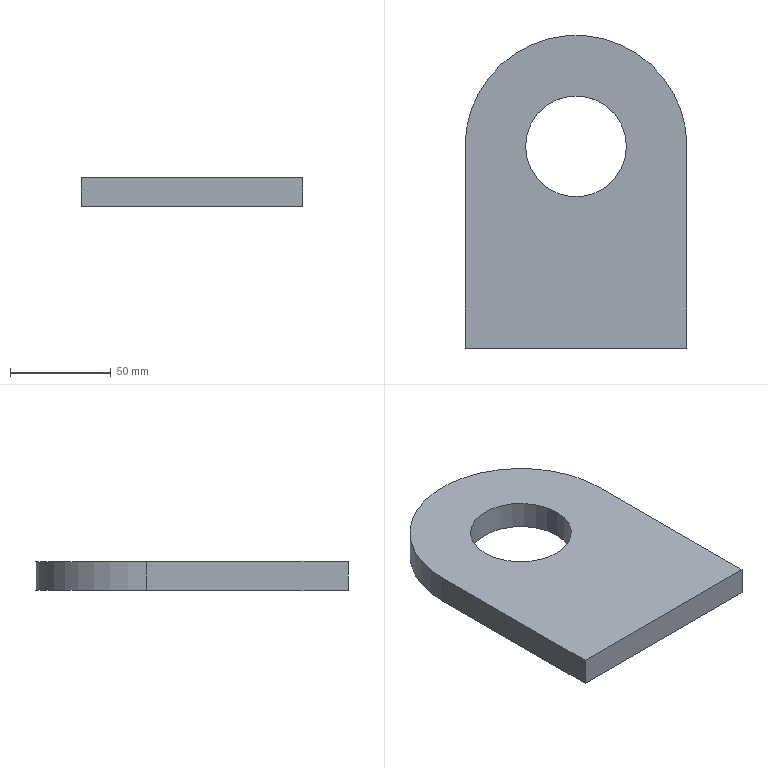Part | SolidWorks | features Extrusion 1 | 1 solid | 8 faces | box 110 x 155 x 14 mm | volume 193034 mm3 | plane 5 | cylinder 3 | commonest cylinder face diameters 50 x2 110 x1
STEP:
#1=CARTESIAN_POINT('',(-25.,0.,14.));
#2=VERTEX_POINT('',#1);
#3=CARTESIAN_POINT('',(25.,0.,14.));
#4=VERTEX_POINT('',#3);
#5=CARTESIAN_POINT('',(0.,0.,14.));
#6=DIRECTION('',(0.,0.,1.));
#7=DIRECTION('',(1.,0.,0.));
#8=AXIS2_PLACEMENT_3D('',#5,#6,#7);
#9=CIRCLE('',#8,25.);
#10=EDGE_CURVE('',#2,#4,#9,.T.);
#11=ORIENTED_EDGE('',*,*,#10,.T.);
#12=CARTESIAN_POINT('',(25.,0.,0.));
#13=VERTEX_POINT('',#12);
#14=CARTESIAN_POINT('',(25.,0.,14.));
#15=DIRECTION('',(0.,0.,-1.));
#16=VECTOR('',#15,1000.);
#17=LINE('',#14,#16);
#18=EDGE_CURVE('',#4,#13,#17,.T.);
#19=ORIENTED_EDGE('',*,*,#18,.T.);
#20=CARTESIAN_POINT('',(-25.,0.,0.));
#21=VERTEX_POINT('',#20);
#22=CARTESIAN_POINT('',(0.,0.,0.));
#23=DIRECTION('',(0.,0.,1.));
#24=DIRECTION('',(1.,0.,0.));
#25=AXIS2_PLACEMENT_3D('',#22,#23,#24);
#26=CIRCLE('',#25,25.);
#27=EDGE_CURVE('',#21,#13,#26,.T.);
#28=ORIENTED_EDGE('',*,*,#27,.F.);
#29=CARTESIAN_POINT('',(-25.,0.,14.));
#30=DIRECTION('',(0.,0.,-1.));
#31=VECTOR('',#30,1000.);
#32=LINE('',#29,#31);
#33=EDGE_CURVE('',#2,#21,#32,.T.);
#34=ORIENTED_EDGE('',*,*,#33,.F.);
#35=EDGE_LOOP('',(#11,#19,#28,#34));
#36=FACE_OUTER_BOUND('',#35,.T.);
#37=CARTESIAN_POINT('',(0.,0.,14.));
#38=DIRECTION('',(0.,0.,-1.));
#39=DIRECTION('',(-1.,0.,0.));
#40=AXIS2_PLACEMENT_3D('',#37,#38,#39);
#41=CYLINDRICAL_SURFACE('',#40,25.);
#42=ADVANCED_FACE('',(#36),#41,.F.);
#43=CARTESIAN_POINT('',(55.,0.,14.));
#44=VERTEX_POINT('',#43);
#45=CARTESIAN_POINT('',(-55.,0.,14.));
#46=VERTEX_POINT('',#45);
#47=CARTESIAN_POINT('',(0.,0.,14.));
#48=DIRECTION('',(0.,0.,1.));
#49=DIRECTION('',(1.,0.,0.));
#50=AXIS2_PLACEMENT_3D('',#47,#48,#49);
#51=CIRCLE('',#50,55.);
#52=EDGE_CURVE('',#44,#46,#51,.T.);
#53=ORIENTED_EDGE('',*,*,#52,.T.);
#54=CARTESIAN_POINT('',(-55.,-100.,14.));
#55=VERTEX_POINT('',#54);
#56=CARTESIAN_POINT('',(-55.,0.,14.));
#57=DIRECTION('',(0.,-1.,0.));
#58=VECTOR('',#57,1000.);
#59=LINE('',#56,#58);
#60=EDGE_CURVE('',#46,#55,#59,.T.);
#61=ORIENTED_EDGE('',*,*,#60,.T.);
#62=CARTESIAN_POINT('',(55.,-100.,14.));
#63=VERTEX_POINT('',#62);
#64=CARTESIAN_POINT('',(-55.,-100.,14.));
#65=DIRECTION('',(1.,0.,0.));
#66=VECTOR('',#65,1000.);
#67=LINE('',#64,#66);
#68=EDGE_CURVE('',#55,#63,#67,.T.);
#69=ORIENTED_EDGE('',*,*,#68,.T.);
#70=CARTESIAN_POINT('',(55.,-100.,14.));
#71=DIRECTION('',(0.,1.,0.));
#72=VECTOR('',#71,1000.);
#73=LINE('',#70,#72);
#74=EDGE_CURVE('',#63,#44,#73,.T.);
#75=ORIENTED_EDGE('',*,*,#74,.T.);
#76=EDGE_LOOP('',(#53,#61,#69,#75));
#77=FACE_OUTER_BOUND('',#76,.T.);
#78=ORIENTED_EDGE('',*,*,#10,.F.);
#79=CARTESIAN_POINT('',(0.,0.,14.));
#80=DIRECTION('',(0.,0.,1.));
#81=DIRECTION('',(1.,0.,0.));
#82=AXIS2_PLACEMENT_3D('',#79,#80,#81);
#83=CIRCLE('',#82,25.);
#84=EDGE_CURVE('',#4,#2,#83,.T.);
#85=ORIENTED_EDGE('',*,*,#84,.F.);
#86=EDGE_LOOP('',(#78,#85));
#87=FACE_BOUND('',#86,.T.);
#88=CARTESIAN_POINT('',(0.,0.,14.));
#89=DIRECTION('',(0.,0.,1.));
#90=DIRECTION('',(1.,0.,0.));
#91=AXIS2_PLACEMENT_3D('',#88,#89,#90);
#92=PLANE('',#91);
#93=ADVANCED_FACE('',(#77,#87),#92,.T.);
#94=CARTESIAN_POINT('',(55.,0.,0.));
#95=VERTEX_POINT('',#94);
#96=CARTESIAN_POINT('',(-55.,0.,0.));
#97=VERTEX_POINT('',#96);
#98=CARTESIAN_POINT('',(0.,0.,0.));
#99=DIRECTION('',(0.,0.,1.));
#100=DIRECTION('',(1.,0.,0.));
#101=AXIS2_PLACEMENT_3D('',#98,#99,#100);
#102=CIRCLE('',#101,55.);
#103=EDGE_CURVE('',#95,#97,#102,.T.);
#104=ORIENTED_EDGE('',*,*,#103,.F.);
#105=CARTESIAN_POINT('',(55.,-100.,0.));
#106=VERTEX_POINT('',#105);
#107=CARTESIAN_POINT('',(55.,-100.,0.));
#108=DIRECTION('',(0.,1.,0.));
#109=VECTOR('',#108,1000.);
#110=LINE('',#107,#109);
#111=EDGE_CURVE('',#106,#95,#110,.T.);
#112=ORIENTED_EDGE('',*,*,#111,.F.);
#113=CARTESIAN_POINT('',(-55.,-100.,0.));
#114=VERTEX_POINT('',#113);
#115=CARTESIAN_POINT('',(-55.,-100.,0.));
#116=DIRECTION('',(1.,0.,0.));
#117=VECTOR('',#116,1000.);
#118=LINE('',#115,#117);
#119=EDGE_CURVE('',#114,#106,#118,.T.);
#120=ORIENTED_EDGE('',*,*,#119,.F.);
#121=CARTESIAN_POINT('',(-55.,0.,0.));
#122=DIRECTION('',(0.,-1.,0.));
#123=VECTOR('',#122,1000.);
#124=LINE('',#121,#123);
#125=EDGE_CURVE('',#97,#114,#124,.T.);
#126=ORIENTED_EDGE('',*,*,#125,.F.);
#127=EDGE_LOOP('',(#104,#112,#120,#126));
#128=FACE_OUTER_BOUND('',#127,.T.);
#129=ORIENTED_EDGE('',*,*,#27,.T.);
#130=CARTESIAN_POINT('',(0.,0.,0.));
#131=DIRECTION('',(0.,0.,1.));
#132=DIRECTION('',(1.,0.,0.));
#133=AXIS2_PLACEMENT_3D('',#130,#131,#132);
#134=CIRCLE('',#133,25.);
#135=EDGE_CURVE('',#13,#21,#134,.T.);
#136=ORIENTED_EDGE('',*,*,#135,.T.);
#137=EDGE_LOOP('',(#129,#136));
#138=FACE_BOUND('',#137,.T.);
#139=CARTESIAN_POINT('',(0.,0.,0.));
#140=DIRECTION('',(0.,0.,1.));
#141=DIRECTION('',(1.,0.,0.));
#142=AXIS2_PLACEMENT_3D('',#139,#140,#141);
#143=PLANE('',#142);
#144=ADVANCED_FACE('',(#128,#138),#143,.F.);
#145=ORIENTED_EDGE('',*,*,#103,.T.);
#146=CARTESIAN_POINT('',(-55.,0.,14.));
#147=DIRECTION('',(0.,0.,-1.));
#148=VECTOR('',#147,1000.);
#149=LINE('',#146,#148);
#150=EDGE_CURVE('',#46,#97,#149,.T.);
#151=ORIENTED_EDGE('',*,*,#150,.F.);
#152=ORIENTED_EDGE('',*,*,#52,.F.);
#153=CARTESIAN_POINT('',(55.,0.,14.));
#154=DIRECTION('',(0.,0.,-1.));
#155=VECTOR('',#154,1000.);
#156=LINE('',#153,#155);
#157=EDGE_CURVE('',#44,#95,#156,.T.);
#158=ORIENTED_EDGE('',*,*,#157,.T.);
#159=EDGE_LOOP('',(#145,#151,#152,#158));
#160=FACE_OUTER_BOUND('',#159,.T.);
#161=CARTESIAN_POINT('',(0.,0.,14.));
#162=DIRECTION('',(0.,0.,-1.));
#163=DIRECTION('',(-1.,0.,0.));
#164=AXIS2_PLACEMENT_3D('',#161,#162,#163);
#165=CYLINDRICAL_SURFACE('',#164,55.);
#166=ADVANCED_FACE('',(#160),#165,.T.);
#167=ORIENTED_EDGE('',*,*,#125,.T.);
#168=CARTESIAN_POINT('',(-55.,-100.,14.));
#169=DIRECTION('',(0.,0.,-1.));
#170=VECTOR('',#169,1000.);
#171=LINE('',#168,#170);
#172=EDGE_CURVE('',#55,#114,#171,.T.);
#173=ORIENTED_EDGE('',*,*,#172,.F.);
#174=ORIENTED_EDGE('',*,*,#60,.F.);
#175=ORIENTED_EDGE('',*,*,#150,.T.);
#176=EDGE_LOOP('',(#167,#173,#174,#175));
#177=FACE_OUTER_BOUND('',#176,.T.);
#178=CARTESIAN_POINT('',(-55.,0.,14.));
#179=DIRECTION('',(1.,0.,0.));
#180=DIRECTION('',(0.,1.,0.));
#181=AXIS2_PLACEMENT_3D('',#178,#179,#180);
#182=PLANE('',#181);
#183=ADVANCED_FACE('',(#177),#182,.F.);
#184=ORIENTED_EDGE('',*,*,#119,.T.);
#185=CARTESIAN_POINT('',(55.,-100.,14.));
#186=DIRECTION('',(0.,0.,-1.));
#187=VECTOR('',#186,1000.);
#188=LINE('',#185,#187);
#189=EDGE_CURVE('',#63,#106,#188,.T.);
#190=ORIENTED_EDGE('',*,*,#189,.F.);
#191=ORIENTED_EDGE('',*,*,#68,.F.);
#192=ORIENTED_EDGE('',*,*,#172,.T.);
#193=EDGE_LOOP('',(#184,#190,#191,#192));
#194=FACE_OUTER_BOUND('',#193,.T.);
#195=CARTESIAN_POINT('',(-55.,-100.,14.));
#196=DIRECTION('',(0.,1.,0.));
#197=DIRECTION('',(0.,0.,1.));
#198=AXIS2_PLACEMENT_3D('',#195,#196,#197);
#199=PLANE('',#198);
#200=ADVANCED_FACE('',(#194),#199,.F.);
#201=ORIENTED_EDGE('',*,*,#111,.T.);
#202=ORIENTED_EDGE('',*,*,#157,.F.);
#203=ORIENTED_EDGE('',*,*,#74,.F.);
#204=ORIENTED_EDGE('',*,*,#189,.T.);
#205=EDGE_LOOP('',(#201,#202,#203,#204));
#206=FACE_OUTER_BOUND('',#205,.T.);
#207=CARTESIAN_POINT('',(55.,-100.,14.));
#208=DIRECTION('',(-1.,0.,0.));
#209=DIRECTION('',(0.,-1.,0.));
#210=AXIS2_PLACEMENT_3D('',#207,#208,#209);
#211=PLANE('',#210);
#212=ADVANCED_FACE('',(#206),#211,.F.);
#213=ORIENTED_EDGE('',*,*,#18,.F.);
#214=ORIENTED_EDGE('',*,*,#84,.T.);
#215=ORIENTED_EDGE('',*,*,#33,.T.);
#216=ORIENTED_EDGE('',*,*,#135,.F.);
#217=EDGE_LOOP('',(#213,#214,#215,#216));
#218=FACE_OUTER_BOUND('',#217,.T.);
#219=CARTESIAN_POINT('',(0.,0.,14.));
#220=DIRECTION('',(0.,0.,-1.));
#221=DIRECTION('',(-1.,0.,0.));
#222=AXIS2_PLACEMENT_3D('',#219,#220,#221);
#223=CYLINDRICAL_SURFACE('',#222,25.);
#224=ADVANCED_FACE('',(#218),#223,.F.);
#225=CLOSED_SHELL('',(#42,#93,#144,#166,#183,#200,#212,#224));
#226=MANIFOLD_SOLID_BREP('',#225);
#227=CARTESIAN_POINT('',(0.,0.,0.));
#228=DIRECTION('',(0.,0.,1.));
#229=DIRECTION('',(1.,0.,0.));
#230=AXIS2_PLACEMENT_3D('',#227,#228,#229);
#231=(LENGTH_UNIT()NAMED_UNIT(*)SI_UNIT(.MILLI.,.METRE.));
#232=UNCERTAINTY_MEASURE_WITH_UNIT(LENGTH_MEASURE(0.00001),#231,'','');
#233=(NAMED_UNIT(*)PLANE_ANGLE_UNIT()SI_UNIT($,.RADIAN.));
#234=(NAMED_UNIT(*)SI_UNIT($,.STERADIAN.)SOLID_ANGLE_UNIT());
#235=(GEOMETRIC_REPRESENTATION_CONTEXT(3)GLOBAL_UNCERTAINTY_ASSIGNED_CONTEXT((#232))GLOBAL_UNIT_ASSIGNED_CONTEXT((#231,#233,#234))REPRESENTATION_CONTEXT('',''));
#236=ADVANCED_BREP_SHAPE_REPRESENTATION('',(#226,#230),#235);